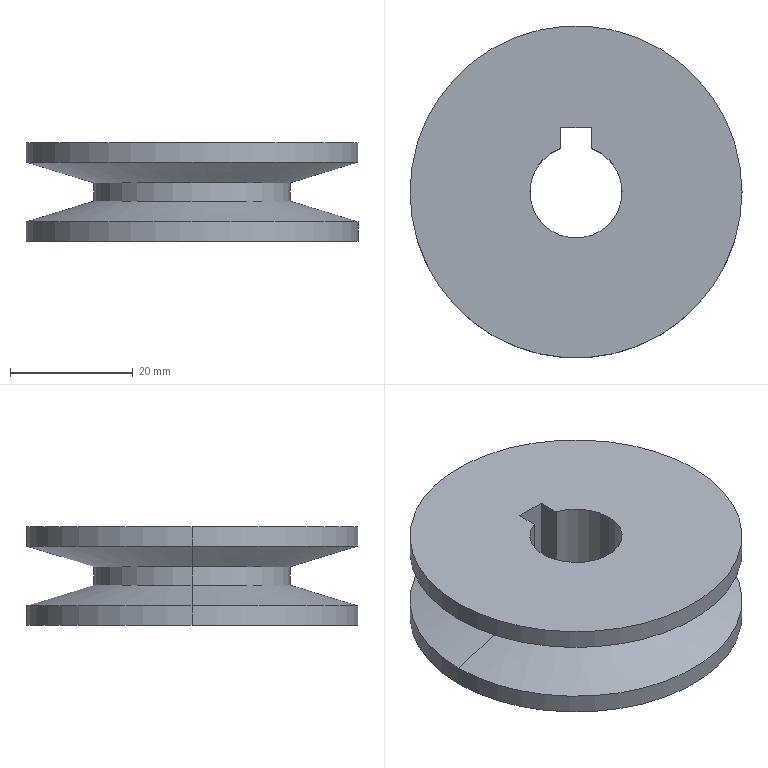Part | SolidWorks | features ICE 2, BaseBody 1 | 1 solid | 18 faces | box 54 x 54 x 16 mm | volume 23688 mm3 | cylinder 9 | plane 5 | cone 4 | commonest cylinder face diameters 54 x4 15 x3 32 x2
STEP:
#1=CARTESIAN_POINT('',(-7.5,0.,0.));
#2=VERTEX_POINT('',#1);
#3=CARTESIAN_POINT('',(7.5,0.,0.));
#4=VERTEX_POINT('',#3);
#5=CARTESIAN_POINT('',(0.,0.,0.));
#6=DIRECTION('',(0.,0.,1.));
#7=DIRECTION('',(1.,0.,0.));
#8=AXIS2_PLACEMENT_3D('',#5,#6,#7);
#9=CIRCLE('',#8,7.5);
#10=EDGE_CURVE('',#2,#4,#9,.T.);
#11=ORIENTED_EDGE('',*,*,#10,.F.);
#12=CARTESIAN_POINT('',(-7.5,0.,16.));
#13=VERTEX_POINT('',#12);
#14=CARTESIAN_POINT('',(-7.5,0.,0.));
#15=DIRECTION('',(0.,0.,1.));
#16=VECTOR('',#15,1000.);
#17=LINE('',#14,#16);
#18=EDGE_CURVE('',#2,#13,#17,.T.);
#19=ORIENTED_EDGE('',*,*,#18,.T.);
#20=CARTESIAN_POINT('',(7.5,0.,16.));
#21=VERTEX_POINT('',#20);
#22=CARTESIAN_POINT('',(0.,0.,16.));
#23=DIRECTION('',(0.,0.,1.));
#24=DIRECTION('',(1.,0.,0.));
#25=AXIS2_PLACEMENT_3D('',#22,#23,#24);
#26=CIRCLE('',#25,7.5);
#27=EDGE_CURVE('',#13,#21,#26,.T.);
#28=ORIENTED_EDGE('',*,*,#27,.T.);
#29=CARTESIAN_POINT('',(7.5,0.,0.));
#30=DIRECTION('',(0.,0.,1.));
#31=VECTOR('',#30,1000.);
#32=LINE('',#29,#31);
#33=EDGE_CURVE('',#4,#21,#32,.T.);
#34=ORIENTED_EDGE('',*,*,#33,.F.);
#35=EDGE_LOOP('',(#11,#19,#28,#34));
#36=FACE_OUTER_BOUND('',#35,.T.);
#37=CARTESIAN_POINT('',(0.,0.,0.));
#38=DIRECTION('',(0.,0.,1.));
#39=DIRECTION('',(1.,0.,0.));
#40=AXIS2_PLACEMENT_3D('',#37,#38,#39);
#41=CYLINDRICAL_SURFACE('',#40,7.5);
#42=ADVANCED_FACE('',(#36),#41,.F.);
#43=CARTESIAN_POINT('',(2.5,7.071,0.));
#44=VERTEX_POINT('',#43);
#45=CARTESIAN_POINT('',(0.,0.,0.));
#46=DIRECTION('',(0.,0.,1.));
#47=DIRECTION('',(1.,0.,0.));
#48=AXIS2_PLACEMENT_3D('',#45,#46,#47);
#49=CIRCLE('',#48,7.5);
#50=EDGE_CURVE('',#4,#44,#49,.T.);
#51=ORIENTED_EDGE('',*,*,#50,.F.);
#52=ORIENTED_EDGE('',*,*,#33,.T.);
#53=CARTESIAN_POINT('',(2.5,7.071,16.));
#54=VERTEX_POINT('',#53);
#55=CARTESIAN_POINT('',(0.,0.,16.));
#56=DIRECTION('',(0.,0.,1.));
#57=DIRECTION('',(1.,0.,0.));
#58=AXIS2_PLACEMENT_3D('',#55,#56,#57);
#59=CIRCLE('',#58,7.5);
#60=EDGE_CURVE('',#21,#54,#59,.T.);
#61=ORIENTED_EDGE('',*,*,#60,.T.);
#62=CARTESIAN_POINT('',(2.5,7.071,0.));
#63=DIRECTION('',(0.,0.,-1.));
#64=VECTOR('',#63,1000.);
#65=LINE('',#62,#64);
#66=EDGE_CURVE('',#54,#44,#65,.T.);
#67=ORIENTED_EDGE('',*,*,#66,.T.);
#68=EDGE_LOOP('',(#51,#52,#61,#67));
#69=FACE_OUTER_BOUND('',#68,.T.);
#70=CARTESIAN_POINT('',(0.,0.,0.));
#71=DIRECTION('',(0.,0.,1.));
#72=DIRECTION('',(1.,0.,0.));
#73=AXIS2_PLACEMENT_3D('',#70,#71,#72);
#74=CYLINDRICAL_SURFACE('',#73,7.5);
#75=ADVANCED_FACE('',(#69),#74,.F.);
#76=CARTESIAN_POINT('',(27.,0.,16.));
#77=VERTEX_POINT('',#76);
#78=CARTESIAN_POINT('',(-27.,0.,16.));
#79=VERTEX_POINT('',#78);
#80=CARTESIAN_POINT('',(0.,0.,16.));
#81=DIRECTION('',(0.,0.,1.));
#82=DIRECTION('',(-1.,0.,0.));
#83=AXIS2_PLACEMENT_3D('',#80,#81,#82);
#84=CIRCLE('',#83,27.);
#85=EDGE_CURVE('',#77,#79,#84,.T.);
#86=ORIENTED_EDGE('',*,*,#85,.F.);
#87=CARTESIAN_POINT('',(27.,0.,12.861));
#88=VERTEX_POINT('',#87);
#89=CARTESIAN_POINT('',(27.,0.,8.));
#90=DIRECTION('',(0.,0.,-1.));
#91=VECTOR('',#90,1000.);
#92=LINE('',#89,#91);
#93=EDGE_CURVE('',#77,#88,#92,.T.);
#94=ORIENTED_EDGE('',*,*,#93,.T.);
#95=CARTESIAN_POINT('',(-27.,0.,12.861));
#96=VERTEX_POINT('',#95);
#97=CARTESIAN_POINT('',(0.,0.,12.861));
#98=DIRECTION('',(0.,0.,1.));
#99=DIRECTION('',(-1.,0.,0.));
#100=AXIS2_PLACEMENT_3D('',#97,#98,#99);
#101=CIRCLE('',#100,27.);
#102=EDGE_CURVE('',#88,#96,#101,.T.);
#103=ORIENTED_EDGE('',*,*,#102,.T.);
#104=CARTESIAN_POINT('',(-27.,0.,8.));
#105=DIRECTION('',(0.,0.,-1.));
#106=VECTOR('',#105,1000.);
#107=LINE('',#104,#106);
#108=EDGE_CURVE('',#79,#96,#107,.T.);
#109=ORIENTED_EDGE('',*,*,#108,.F.);
#110=EDGE_LOOP('',(#86,#94,#103,#109));
#111=FACE_OUTER_BOUND('',#110,.T.);
#112=CARTESIAN_POINT('',(0.,0.,8.));
#113=DIRECTION('',(0.,0.,-1.));
#114=DIRECTION('',(-1.,0.,0.));
#115=AXIS2_PLACEMENT_3D('',#112,#113,#114);
#116=CYLINDRICAL_SURFACE('',#115,27.);
#117=ADVANCED_FACE('',(#111),#116,.T.);
#118=CARTESIAN_POINT('',(16.,0.,9.498));
#119=VERTEX_POINT('',#118);
#120=CARTESIAN_POINT('',(-16.,0.,9.498));
#121=VERTEX_POINT('',#120);
#122=CARTESIAN_POINT('',(0.,0.,9.498));
#123=DIRECTION('',(0.,0.,1.));
#124=DIRECTION('',(0.,1.,0.));
#125=AXIS2_PLACEMENT_3D('',#122,#123,#124);
#126=CIRCLE('',#125,16.);
#127=EDGE_CURVE('',#119,#121,#126,.T.);
#128=ORIENTED_EDGE('',*,*,#127,.T.);
#129=CARTESIAN_POINT('',(-27.,0.,12.861));
#130=DIRECTION('',(-0.9563,0.,0.2924));
#131=VECTOR('',#130,1000.);
#132=LINE('',#129,#131);
#133=EDGE_CURVE('',#121,#96,#132,.T.);
#134=ORIENTED_EDGE('',*,*,#133,.T.);
#135=ORIENTED_EDGE('',*,*,#102,.F.);
#136=CARTESIAN_POINT('',(27.,0.,12.861));
#137=DIRECTION('',(0.9563,0.,0.2924));
#138=VECTOR('',#137,1000.);
#139=LINE('',#136,#138);
#140=EDGE_CURVE('',#119,#88,#139,.T.);
#141=ORIENTED_EDGE('',*,*,#140,.F.);
#142=EDGE_LOOP('',(#128,#134,#135,#141));
#143=FACE_OUTER_BOUND('',#142,.T.);
#144=CARTESIAN_POINT('',(0.,0.,12.861));
#145=DIRECTION('',(0.,0.,1.));
#146=DIRECTION('',(1.,0.,0.));
#147=AXIS2_PLACEMENT_3D('',#144,#145,#146);
#148=CONICAL_SURFACE('',#147,27.,1.274);
#149=ADVANCED_FACE('',(#143),#148,.T.);
#150=CARTESIAN_POINT('',(16.,0.,6.502));
#151=VERTEX_POINT('',#150);
#152=CARTESIAN_POINT('',(-16.,0.,6.502));
#153=VERTEX_POINT('',#152);
#154=CARTESIAN_POINT('',(0.,0.,6.502));
#155=DIRECTION('',(0.,0.,1.));
#156=DIRECTION('',(1.,0.,0.));
#157=AXIS2_PLACEMENT_3D('',#154,#155,#156);
#158=CIRCLE('',#157,16.);
#159=EDGE_CURVE('',#151,#153,#158,.T.);
#160=ORIENTED_EDGE('',*,*,#159,.T.);
#161=CARTESIAN_POINT('',(-16.,0.,8.));
#162=DIRECTION('',(0.,0.,1.));
#163=VECTOR('',#162,1000.);
#164=LINE('',#161,#163);
#165=EDGE_CURVE('',#153,#121,#164,.T.);
#166=ORIENTED_EDGE('',*,*,#165,.T.);
#167=ORIENTED_EDGE('',*,*,#127,.F.);
#168=CARTESIAN_POINT('',(16.,0.,8.));
#169=DIRECTION('',(0.,0.,1.));
#170=VECTOR('',#169,1000.);
#171=LINE('',#168,#170);
#172=EDGE_CURVE('',#151,#119,#171,.T.);
#173=ORIENTED_EDGE('',*,*,#172,.F.);
#174=EDGE_LOOP('',(#160,#166,#167,#173));
#175=FACE_OUTER_BOUND('',#174,.T.);
#176=CARTESIAN_POINT('',(0.,0.,8.));
#177=DIRECTION('',(0.,0.,1.));
#178=DIRECTION('',(1.,0.,0.));
#179=AXIS2_PLACEMENT_3D('',#176,#177,#178);
#180=CYLINDRICAL_SURFACE('',#179,16.);
#181=ADVANCED_FACE('',(#175),#180,.T.);
#182=ORIENTED_EDGE('',*,*,#159,.F.);
#183=CARTESIAN_POINT('',(27.,0.,3.139));
#184=VERTEX_POINT('',#183);
#185=CARTESIAN_POINT('',(27.,0.,3.139));
#186=DIRECTION('',(0.9563,0.,-0.2924));
#187=VECTOR('',#186,1000.);
#188=LINE('',#185,#187);
#189=EDGE_CURVE('',#151,#184,#188,.T.);
#190=ORIENTED_EDGE('',*,*,#189,.T.);
#191=CARTESIAN_POINT('',(-27.,0.,3.139));
#192=VERTEX_POINT('',#191);
#193=CARTESIAN_POINT('',(0.,0.,3.139));
#194=DIRECTION('',(0.,0.,1.));
#195=DIRECTION('',(0.,1.,0.));
#196=AXIS2_PLACEMENT_3D('',#193,#194,#195);
#197=CIRCLE('',#196,27.);
#198=EDGE_CURVE('',#184,#192,#197,.T.);
#199=ORIENTED_EDGE('',*,*,#198,.T.);
#200=CARTESIAN_POINT('',(-27.,0.,3.139));
#201=DIRECTION('',(-0.9563,0.,-0.2924));
#202=VECTOR('',#201,1000.);
#203=LINE('',#200,#202);
#204=EDGE_CURVE('',#153,#192,#203,.T.);
#205=ORIENTED_EDGE('',*,*,#204,.F.);
#206=EDGE_LOOP('',(#182,#190,#199,#205));
#207=FACE_OUTER_BOUND('',#206,.T.);
#208=CARTESIAN_POINT('',(0.,0.,3.139));
#209=DIRECTION('',(0.,0.,-1.));
#210=DIRECTION('',(-1.,0.,0.));
#211=AXIS2_PLACEMENT_3D('',#208,#209,#210);
#212=CONICAL_SURFACE('',#211,27.,1.274);
#213=ADVANCED_FACE('',(#207),#212,.T.);
#214=ORIENTED_EDGE('',*,*,#198,.F.);
#215=CARTESIAN_POINT('',(27.,0.,0.));
#216=VERTEX_POINT('',#215);
#217=CARTESIAN_POINT('',(27.,0.,8.));
#218=DIRECTION('',(0.,0.,-1.));
#219=VECTOR('',#218,1000.);
#220=LINE('',#217,#219);
#221=EDGE_CURVE('',#184,#216,#220,.T.);
#222=ORIENTED_EDGE('',*,*,#221,.T.);
#223=CARTESIAN_POINT('',(-27.,0.,0.));
#224=VERTEX_POINT('',#223);
#225=CARTESIAN_POINT('',(0.,0.,0.));
#226=DIRECTION('',(0.,0.,1.));
#227=DIRECTION('',(-1.,0.,0.));
#228=AXIS2_PLACEMENT_3D('',#225,#226,#227);
#229=CIRCLE('',#228,27.);
#230=EDGE_CURVE('',#216,#224,#229,.T.);
#231=ORIENTED_EDGE('',*,*,#230,.T.);
#232=CARTESIAN_POINT('',(-27.,0.,8.));
#233=DIRECTION('',(0.,0.,-1.));
#234=VECTOR('',#233,1000.);
#235=LINE('',#232,#234);
#236=EDGE_CURVE('',#192,#224,#235,.T.);
#237=ORIENTED_EDGE('',*,*,#236,.F.);
#238=EDGE_LOOP('',(#214,#222,#231,#237));
#239=FACE_OUTER_BOUND('',#238,.T.);
#240=CARTESIAN_POINT('',(0.,0.,8.));
#241=DIRECTION('',(0.,0.,-1.));
#242=DIRECTION('',(-1.,0.,0.));
#243=AXIS2_PLACEMENT_3D('',#240,#241,#242);
#244=CYLINDRICAL_SURFACE('',#243,27.);
#245=ADVANCED_FACE('',(#239),#244,.T.);
#246=CARTESIAN_POINT('',(-2.5,10.5,16.));
#247=VERTEX_POINT('',#246);
#248=CARTESIAN_POINT('',(-2.5,7.071,16.));
#249=VERTEX_POINT('',#248);
#250=CARTESIAN_POINT('',(-2.5,10.5,16.));
#251=DIRECTION('',(0.,-1.,0.));
#252=VECTOR('',#251,1000.);
#253=LINE('',#250,#252);
#254=EDGE_CURVE('',#247,#249,#253,.T.);
#255=ORIENTED_EDGE('',*,*,#254,.F.);
#256=CARTESIAN_POINT('',(2.5,10.5,16.));
#257=VERTEX_POINT('',#256);
#258=CARTESIAN_POINT('',(-2.5,10.5,16.));
#259=DIRECTION('',(-1.,0.,0.));
#260=VECTOR('',#259,1000.);
#261=LINE('',#258,#260);
#262=EDGE_CURVE('',#257,#247,#261,.T.);
#263=ORIENTED_EDGE('',*,*,#262,.F.);
#264=CARTESIAN_POINT('',(2.5,10.5,16.));
#265=DIRECTION('',(0.,1.,0.));
#266=VECTOR('',#265,1000.);
#267=LINE('',#264,#266);
#268=EDGE_CURVE('',#54,#257,#267,.T.);
#269=ORIENTED_EDGE('',*,*,#268,.F.);
#270=ORIENTED_EDGE('',*,*,#60,.F.);
#271=ORIENTED_EDGE('',*,*,#27,.F.);
#272=CARTESIAN_POINT('',(0.,0.,16.));
#273=DIRECTION('',(0.,0.,1.));
#274=DIRECTION('',(1.,0.,0.));
#275=AXIS2_PLACEMENT_3D('',#272,#273,#274);
#276=CIRCLE('',#275,7.5);
#277=EDGE_CURVE('',#249,#13,#276,.T.);
#278=ORIENTED_EDGE('',*,*,#277,.F.);
#279=EDGE_LOOP('',(#255,#263,#269,#270,#271,#278));
#280=FACE_BOUND('',#279,.T.);
#281=CARTESIAN_POINT('',(0.,0.,16.));
#282=DIRECTION('',(0.,0.,1.));
#283=DIRECTION('',(-1.,0.,0.));
#284=AXIS2_PLACEMENT_3D('',#281,#282,#283);
#285=CIRCLE('',#284,27.);
#286=EDGE_CURVE('',#79,#77,#285,.T.);
#287=ORIENTED_EDGE('',*,*,#286,.T.);
#288=ORIENTED_EDGE('',*,*,#85,.T.);
#289=EDGE_LOOP('',(#287,#288));
#290=FACE_OUTER_BOUND('',#289,.T.);
#291=CARTESIAN_POINT('',(0.,13.5,16.));
#292=DIRECTION('',(0.,0.,1.));
#293=DIRECTION('',(1.,0.,0.));
#294=AXIS2_PLACEMENT_3D('',#291,#292,#293);
#295=PLANE('',#294);
#296=ADVANCED_FACE('',(#280,#290),#295,.T.);
#297=ORIENTED_EDGE('',*,*,#93,.F.);
#298=ORIENTED_EDGE('',*,*,#286,.F.);
#299=ORIENTED_EDGE('',*,*,#108,.T.);
#300=CARTESIAN_POINT('',(0.,0.,12.861));
#301=DIRECTION('',(0.,0.,1.));
#302=DIRECTION('',(-1.,0.,0.));
#303=AXIS2_PLACEMENT_3D('',#300,#301,#302);
#304=CIRCLE('',#303,27.);
#305=EDGE_CURVE('',#96,#88,#304,.T.);
#306=ORIENTED_EDGE('',*,*,#305,.T.);
#307=EDGE_LOOP('',(#297,#298,#299,#306));
#308=FACE_OUTER_BOUND('',#307,.T.);
#309=CARTESIAN_POINT('',(0.,0.,8.));
#310=DIRECTION('',(0.,0.,-1.));
#311=DIRECTION('',(-1.,0.,0.));
#312=AXIS2_PLACEMENT_3D('',#309,#310,#311);
#313=CYLINDRICAL_SURFACE('',#312,27.);
#314=ADVANCED_FACE('',(#308),#313,.T.);
#315=ORIENTED_EDGE('',*,*,#133,.F.);
#316=CARTESIAN_POINT('',(0.,0.,9.498));
#317=DIRECTION('',(0.,0.,1.));
#318=DIRECTION('',(0.,1.,0.));
#319=AXIS2_PLACEMENT_3D('',#316,#317,#318);
#320=CIRCLE('',#319,16.);
#321=EDGE_CURVE('',#121,#119,#320,.T.);
#322=ORIENTED_EDGE('',*,*,#321,.T.);
#323=ORIENTED_EDGE('',*,*,#140,.T.);
#324=ORIENTED_EDGE('',*,*,#305,.F.);
#325=EDGE_LOOP('',(#315,#322,#323,#324));
#326=FACE_OUTER_BOUND('',#325,.T.);
#327=CARTESIAN_POINT('',(0.,0.,12.861));
#328=DIRECTION('',(0.,0.,1.));
#329=DIRECTION('',(1.,0.,0.));
#330=AXIS2_PLACEMENT_3D('',#327,#328,#329);
#331=CONICAL_SURFACE('',#330,27.,1.274);
#332=ADVANCED_FACE('',(#326),#331,.T.);
#333=ORIENTED_EDGE('',*,*,#165,.F.);
#334=CARTESIAN_POINT('',(0.,0.,6.502));
#335=DIRECTION('',(0.,0.,1.));
#336=DIRECTION('',(1.,0.,0.));
#337=AXIS2_PLACEMENT_3D('',#334,#335,#336);
#338=CIRCLE('',#337,16.);
#339=EDGE_CURVE('',#153,#151,#338,.T.);
#340=ORIENTED_EDGE('',*,*,#339,.T.);
#341=ORIENTED_EDGE('',*,*,#172,.T.);
#342=ORIENTED_EDGE('',*,*,#321,.F.);
#343=EDGE_LOOP('',(#333,#340,#341,#342));
#344=FACE_OUTER_BOUND('',#343,.T.);
#345=CARTESIAN_POINT('',(0.,0.,8.));
#346=DIRECTION('',(0.,0.,1.));
#347=DIRECTION('',(1.,0.,0.));
#348=AXIS2_PLACEMENT_3D('',#345,#346,#347);
#349=CYLINDRICAL_SURFACE('',#348,16.);
#350=ADVANCED_FACE('',(#344),#349,.T.);
#351=ORIENTED_EDGE('',*,*,#189,.F.);
#352=ORIENTED_EDGE('',*,*,#339,.F.);
#353=ORIENTED_EDGE('',*,*,#204,.T.);
#354=CARTESIAN_POINT('',(0.,0.,3.139));
#355=DIRECTION('',(0.,0.,1.));
#356=DIRECTION('',(0.,1.,0.));
#357=AXIS2_PLACEMENT_3D('',#354,#355,#356);
#358=CIRCLE('',#357,27.);
#359=EDGE_CURVE('',#192,#184,#358,.T.);
#360=ORIENTED_EDGE('',*,*,#359,.T.);
#361=EDGE_LOOP('',(#351,#352,#353,#360));
#362=FACE_OUTER_BOUND('',#361,.T.);
#363=CARTESIAN_POINT('',(0.,0.,3.139));
#364=DIRECTION('',(0.,0.,-1.));
#365=DIRECTION('',(-1.,0.,0.));
#366=AXIS2_PLACEMENT_3D('',#363,#364,#365);
#367=CONICAL_SURFACE('',#366,27.,1.274);
#368=ADVANCED_FACE('',(#362),#367,.T.);
#369=ORIENTED_EDGE('',*,*,#221,.F.);
#370=ORIENTED_EDGE('',*,*,#359,.F.);
#371=ORIENTED_EDGE('',*,*,#236,.T.);
#372=CARTESIAN_POINT('',(0.,0.,0.));
#373=DIRECTION('',(0.,0.,1.));
#374=DIRECTION('',(-1.,0.,0.));
#375=AXIS2_PLACEMENT_3D('',#372,#373,#374);
#376=CIRCLE('',#375,27.);
#377=EDGE_CURVE('',#224,#216,#376,.T.);
#378=ORIENTED_EDGE('',*,*,#377,.T.);
#379=EDGE_LOOP('',(#369,#370,#371,#378));
#380=FACE_OUTER_BOUND('',#379,.T.);
#381=CARTESIAN_POINT('',(0.,0.,8.));
#382=DIRECTION('',(0.,0.,-1.));
#383=DIRECTION('',(-1.,0.,0.));
#384=AXIS2_PLACEMENT_3D('',#381,#382,#383);
#385=CYLINDRICAL_SURFACE('',#384,27.);
#386=ADVANCED_FACE('',(#380),#385,.T.);
#387=CARTESIAN_POINT('',(-2.5,10.5,0.));
#388=VERTEX_POINT('',#387);
#389=CARTESIAN_POINT('',(-2.5,7.071,0.));
#390=VERTEX_POINT('',#389);
#391=CARTESIAN_POINT('',(-2.5,10.5,0.));
#392=DIRECTION('',(0.,-1.,0.));
#393=VECTOR('',#392,1000.);
#394=LINE('',#391,#393);
#395=EDGE_CURVE('',#388,#390,#394,.T.);
#396=ORIENTED_EDGE('',*,*,#395,.T.);
#397=CARTESIAN_POINT('',(0.,0.,0.));
#398=DIRECTION('',(0.,0.,1.));
#399=DIRECTION('',(1.,0.,0.));
#400=AXIS2_PLACEMENT_3D('',#397,#398,#399);
#401=CIRCLE('',#400,7.5);
#402=EDGE_CURVE('',#390,#2,#401,.T.);
#403=ORIENTED_EDGE('',*,*,#402,.T.);
#404=ORIENTED_EDGE('',*,*,#10,.T.);
#405=ORIENTED_EDGE('',*,*,#50,.T.);
#406=CARTESIAN_POINT('',(2.5,10.5,0.));
#407=VERTEX_POINT('',#406);
#408=CARTESIAN_POINT('',(2.5,10.5,0.));
#409=DIRECTION('',(0.,1.,0.));
#410=VECTOR('',#409,1000.);
#411=LINE('',#408,#410);
#412=EDGE_CURVE('',#44,#407,#411,.T.);
#413=ORIENTED_EDGE('',*,*,#412,.T.);
#414=CARTESIAN_POINT('',(-2.5,10.5,0.));
#415=DIRECTION('',(-1.,0.,0.));
#416=VECTOR('',#415,1000.);
#417=LINE('',#414,#416);
#418=EDGE_CURVE('',#407,#388,#417,.T.);
#419=ORIENTED_EDGE('',*,*,#418,.T.);
#420=EDGE_LOOP('',(#396,#403,#404,#405,#413,#419));
#421=FACE_BOUND('',#420,.T.);
#422=ORIENTED_EDGE('',*,*,#377,.F.);
#423=ORIENTED_EDGE('',*,*,#230,.F.);
#424=EDGE_LOOP('',(#422,#423));
#425=FACE_OUTER_BOUND('',#424,.T.);
#426=CARTESIAN_POINT('',(0.,13.5,0.));
#427=DIRECTION('',(0.,0.,-1.));
#428=DIRECTION('',(-1.,0.,0.));
#429=AXIS2_PLACEMENT_3D('',#426,#427,#428);
#430=PLANE('',#429);
#431=ADVANCED_FACE('',(#421,#425),#430,.T.);
#432=ORIENTED_EDGE('',*,*,#18,.F.);
#433=ORIENTED_EDGE('',*,*,#402,.F.);
#434=CARTESIAN_POINT('',(-2.5,7.071,0.));
#435=DIRECTION('',(0.,0.,1.));
#436=VECTOR('',#435,1000.);
#437=LINE('',#434,#436);
#438=EDGE_CURVE('',#390,#249,#437,.T.);
#439=ORIENTED_EDGE('',*,*,#438,.T.);
#440=ORIENTED_EDGE('',*,*,#277,.T.);
#441=EDGE_LOOP('',(#432,#433,#439,#440));
#442=FACE_OUTER_BOUND('',#441,.T.);
#443=CARTESIAN_POINT('',(0.,0.,0.));
#444=DIRECTION('',(0.,0.,1.));
#445=DIRECTION('',(1.,0.,0.));
#446=AXIS2_PLACEMENT_3D('',#443,#444,#445);
#447=CYLINDRICAL_SURFACE('',#446,7.5);
#448=ADVANCED_FACE('',(#442),#447,.F.);
#449=ORIENTED_EDGE('',*,*,#395,.F.);
#450=CARTESIAN_POINT('',(-2.5,10.5,0.));
#451=DIRECTION('',(0.,0.,1.));
#452=VECTOR('',#451,1000.);
#453=LINE('',#450,#452);
#454=EDGE_CURVE('',#388,#247,#453,.T.);
#455=ORIENTED_EDGE('',*,*,#454,.T.);
#456=ORIENTED_EDGE('',*,*,#254,.T.);
#457=ORIENTED_EDGE('',*,*,#438,.F.);
#458=EDGE_LOOP('',(#449,#455,#456,#457));
#459=FACE_OUTER_BOUND('',#458,.T.);
#460=CARTESIAN_POINT('',(-2.5,10.5,0.));
#461=DIRECTION('',(-1.,0.,0.));
#462=DIRECTION('',(0.,-1.,0.));
#463=AXIS2_PLACEMENT_3D('',#460,#461,#462);
#464=PLANE('',#463);
#465=ADVANCED_FACE('',(#459),#464,.F.);
#466=ORIENTED_EDGE('',*,*,#268,.T.);
#467=CARTESIAN_POINT('',(2.5,10.5,0.));
#468=DIRECTION('',(0.,0.,1.));
#469=VECTOR('',#468,1000.);
#470=LINE('',#467,#469);
#471=EDGE_CURVE('',#407,#257,#470,.T.);
#472=ORIENTED_EDGE('',*,*,#471,.F.);
#473=ORIENTED_EDGE('',*,*,#412,.F.);
#474=ORIENTED_EDGE('',*,*,#66,.F.);
#475=EDGE_LOOP('',(#466,#472,#473,#474));
#476=FACE_OUTER_BOUND('',#475,.T.);
#477=CARTESIAN_POINT('',(2.5,10.5,0.));
#478=DIRECTION('',(1.,0.,0.));
#479=DIRECTION('',(0.,1.,0.));
#480=AXIS2_PLACEMENT_3D('',#477,#478,#479);
#481=PLANE('',#480);
#482=ADVANCED_FACE('',(#476),#481,.F.);
#483=ORIENTED_EDGE('',*,*,#262,.T.);
#484=ORIENTED_EDGE('',*,*,#454,.F.);
#485=ORIENTED_EDGE('',*,*,#418,.F.);
#486=ORIENTED_EDGE('',*,*,#471,.T.);
#487=EDGE_LOOP('',(#483,#484,#485,#486));
#488=FACE_OUTER_BOUND('',#487,.T.);
#489=CARTESIAN_POINT('',(-2.5,10.5,0.));
#490=DIRECTION('',(0.,1.,0.));
#491=DIRECTION('',(0.,0.,1.));
#492=AXIS2_PLACEMENT_3D('',#489,#490,#491);
#493=PLANE('',#492);
#494=ADVANCED_FACE('',(#488),#493,.F.);
#495=CLOSED_SHELL('',(#42,#75,#117,#149,#181,#213,#245,#296,#314,#332,#350,#368,#386,#431,#448,#465,#482,#494));
#496=MANIFOLD_SOLID_BREP('',#495);
#497=CARTESIAN_POINT('',(0.,0.,0.));
#498=DIRECTION('',(0.,0.,1.));
#499=DIRECTION('',(1.,0.,0.));
#500=AXIS2_PLACEMENT_3D('',#497,#498,#499);
#501=(LENGTH_UNIT()NAMED_UNIT(*)SI_UNIT(.MILLI.,.METRE.));
#502=UNCERTAINTY_MEASURE_WITH_UNIT(LENGTH_MEASURE(0.00001),#501,'','');
#503=(NAMED_UNIT(*)PLANE_ANGLE_UNIT()SI_UNIT($,.RADIAN.));
#504=(NAMED_UNIT(*)SI_UNIT($,.STERADIAN.)SOLID_ANGLE_UNIT());
#505=(GEOMETRIC_REPRESENTATION_CONTEXT(3)GLOBAL_UNCERTAINTY_ASSIGNED_CONTEXT((#502))GLOBAL_UNIT_ASSIGNED_CONTEXT((#501,#503,#504))REPRESENTATION_CONTEXT('',''));
#506=ADVANCED_BREP_SHAPE_REPRESENTATION('',(#496,#500),#505);